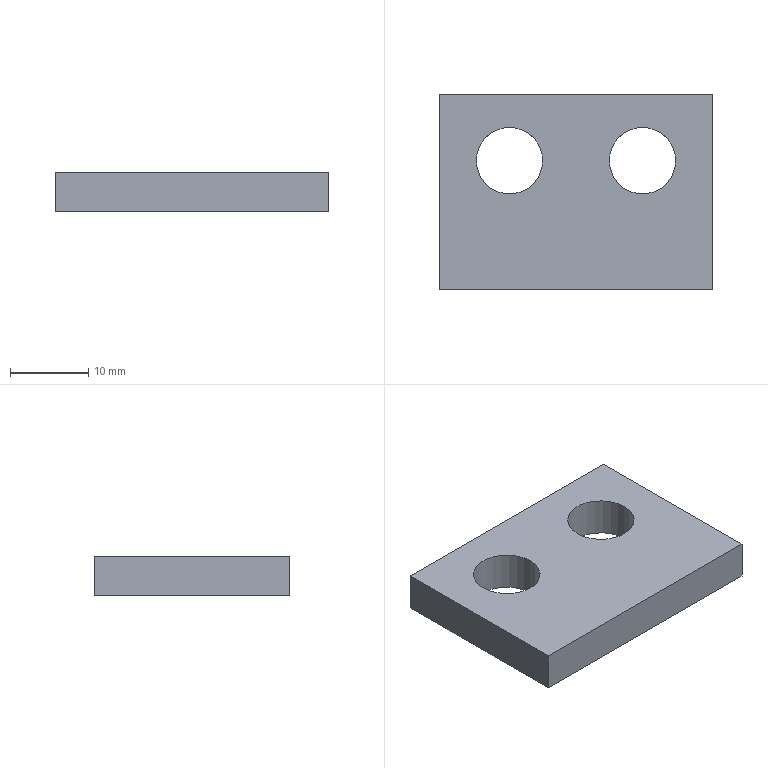Part | NX | features 25 2 | 1 solid | 141 faces | box 35 x 25 x 5 mm | volume 3805 mm3 | plane 102 | spline 37 | cylinder 2 | commonest cylinder face diameters 8.5 x2